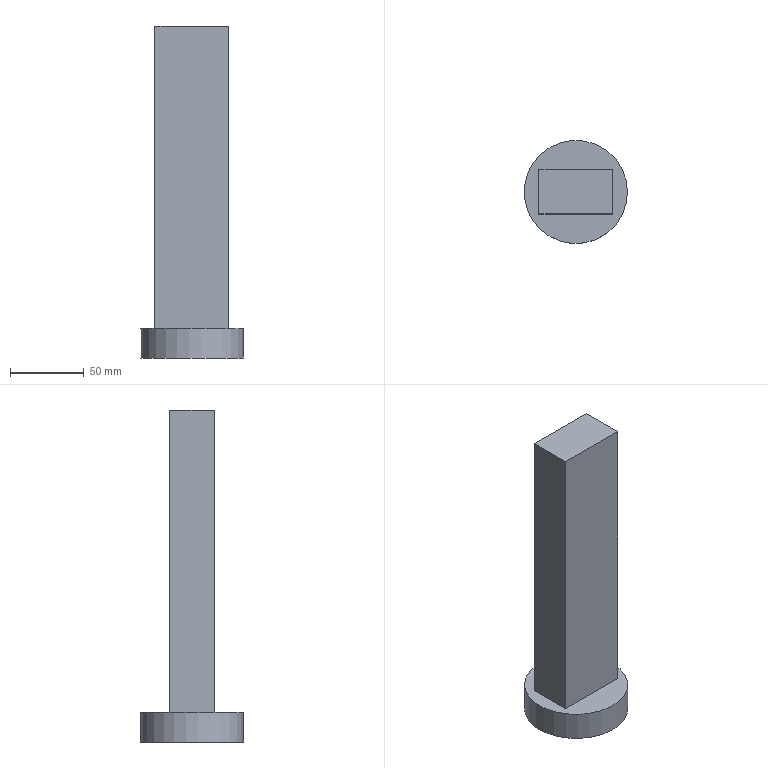Part | NX | features solid 2 | 1 solid | 8 faces | box 70 x 70 x 225 mm | volume 384469 mm3 | plane 7 | cylinder 1 | commonest cylinder face diameters 70 x1
STEP:
#1=CARTESIAN_POINT('',(980.,-425.,0.));
#2=VERTEX_POINT('',#1);
#3=CARTESIAN_POINT('',(945.,-425.,0.));
#4=DIRECTION('',(0.,0.,1.));
#5=DIRECTION('',(1.,0.,0.));
#6=AXIS2_PLACEMENT_3D('',#3,#4,#5);
#7=CIRCLE('',#6,35.);
#8=EDGE_CURVE('',#2,#2,#7,.T.);
#9=ORIENTED_EDGE('',*,*,#8,.F.);
#10=EDGE_LOOP('',(#9));
#11=FACE_BOUND('',#10,.T.);
#12=CARTESIAN_POINT('',(985.,-425.,0.));
#13=DIRECTION('',(0.,0.,1.));
#14=DIRECTION('',(1.,0.,0.));
#15=AXIS2_PLACEMENT_3D('',#12,#13,#14);
#16=PLANE('',#15);
#17=ADVANCED_FACE('',(#11),#16,.F.);
#18=ORIENTED_EDGE('',*,*,#8,.T.);
#19=EDGE_LOOP('',(#18));
#20=FACE_BOUND('',#19,.T.);
#21=CARTESIAN_POINT('',(980.,-425.,20.));
#22=VERTEX_POINT('',#21);
#23=CARTESIAN_POINT('',(945.,-425.,20.));
#24=DIRECTION('',(0.,0.,1.));
#25=DIRECTION('',(1.,0.,0.));
#26=AXIS2_PLACEMENT_3D('',#23,#24,#25);
#27=CIRCLE('',#26,35.);
#28=EDGE_CURVE('',#22,#22,#27,.T.);
#29=ORIENTED_EDGE('',*,*,#28,.F.);
#30=EDGE_LOOP('',(#29));
#31=FACE_BOUND('',#30,.T.);
#32=CARTESIAN_POINT('',(945.,-425.,30.));
#33=DIRECTION('',(0.,0.,1.));
#34=DIRECTION('',(1.,0.,0.));
#35=AXIS2_PLACEMENT_3D('',#32,#33,#34);
#36=CYLINDRICAL_SURFACE('',#35,35.);
#37=ADVANCED_FACE('',(#20,#31),#36,.T.);
#38=ORIENTED_EDGE('',*,*,#28,.T.);
#39=EDGE_LOOP('',(#38));
#40=FACE_BOUND('',#39,.T.);
#41=CARTESIAN_POINT('',(970.,-410.,20.));
#42=VERTEX_POINT('',#41);
#43=CARTESIAN_POINT('',(970.,-440.,20.));
#44=VERTEX_POINT('',#43);
#45=CARTESIAN_POINT('',(970.,-425.,20.));
#46=DIRECTION('',(0.,-1.,0.));
#47=VECTOR('',#46,1000.);
#48=LINE('',#45,#47);
#49=EDGE_CURVE('',#42,#44,#48,.T.);
#50=ORIENTED_EDGE('',*,*,#49,.T.);
#51=CARTESIAN_POINT('',(920.,-440.,20.));
#52=VERTEX_POINT('',#51);
#53=CARTESIAN_POINT('',(525.,-440.,20.));
#54=DIRECTION('',(-1.,0.,0.));
#55=VECTOR('',#54,1000.);
#56=LINE('',#53,#55);
#57=EDGE_CURVE('',#44,#52,#56,.T.);
#58=ORIENTED_EDGE('',*,*,#57,.T.);
#59=CARTESIAN_POINT('',(920.,-410.,20.));
#60=VERTEX_POINT('',#59);
#61=CARTESIAN_POINT('',(920.,-410.,20.));
#62=DIRECTION('',(0.,-1.,0.));
#63=VECTOR('',#62,1000.);
#64=LINE('',#61,#63);
#65=EDGE_CURVE('',#60,#52,#64,.T.);
#66=ORIENTED_EDGE('',*,*,#65,.F.);
#67=CARTESIAN_POINT('',(525.,-410.,20.));
#68=DIRECTION('',(-1.,0.,0.));
#69=VECTOR('',#68,1000.);
#70=LINE('',#67,#69);
#71=EDGE_CURVE('',#42,#60,#70,.T.);
#72=ORIENTED_EDGE('',*,*,#71,.F.);
#73=EDGE_LOOP('',(#50,#58,#66,#72));
#74=FACE_BOUND('',#73,.T.);
#75=CARTESIAN_POINT('',(985.,-425.,20.));
#76=DIRECTION('',(0.,0.,1.));
#77=DIRECTION('',(1.,0.,0.));
#78=AXIS2_PLACEMENT_3D('',#75,#76,#77);
#79=PLANE('',#78);
#80=ADVANCED_FACE('',(#40,#74),#79,.T.);
#81=CARTESIAN_POINT('',(970.,-410.,225.));
#82=VERTEX_POINT('',#81);
#83=CARTESIAN_POINT('',(970.,-410.,155.));
#84=DIRECTION('',(0.,0.,-1.));
#85=VECTOR('',#84,1000.);
#86=LINE('',#83,#85);
#87=EDGE_CURVE('',#82,#42,#86,.T.);
#88=ORIENTED_EDGE('',*,*,#87,.F.);
#89=CARTESIAN_POINT('',(970.,-440.,225.));
#90=VERTEX_POINT('',#89);
#91=CARTESIAN_POINT('',(970.,-410.,225.));
#92=DIRECTION('',(0.,-1.,0.));
#93=VECTOR('',#92,1000.);
#94=LINE('',#91,#93);
#95=EDGE_CURVE('',#82,#90,#94,.T.);
#96=ORIENTED_EDGE('',*,*,#95,.T.);
#97=CARTESIAN_POINT('',(970.,-440.,155.));
#98=DIRECTION('',(0.,0.,-1.));
#99=VECTOR('',#98,1000.);
#100=LINE('',#97,#99);
#101=EDGE_CURVE('',#90,#44,#100,.T.);
#102=ORIENTED_EDGE('',*,*,#101,.T.);
#103=ORIENTED_EDGE('',*,*,#49,.F.);
#104=EDGE_LOOP('',(#88,#96,#102,#103));
#105=FACE_BOUND('',#104,.T.);
#106=CARTESIAN_POINT('',(970.,-410.,365.));
#107=DIRECTION('',(-1.,0.,0.));
#108=DIRECTION('',(0.,-1.,0.));
#109=AXIS2_PLACEMENT_3D('',#106,#107,#108);
#110=PLANE('',#109);
#111=ADVANCED_FACE('',(#105),#110,.F.);
#112=CARTESIAN_POINT('',(920.,-440.,225.));
#113=VERTEX_POINT('',#112);
#114=CARTESIAN_POINT('',(920.,-440.,325.));
#115=DIRECTION('',(0.,0.,-1.));
#116=VECTOR('',#115,1000.);
#117=LINE('',#114,#116);
#118=EDGE_CURVE('',#113,#52,#117,.T.);
#119=ORIENTED_EDGE('',*,*,#118,.F.);
#120=CARTESIAN_POINT('',(920.,-410.,225.));
#121=VERTEX_POINT('',#120);
#122=CARTESIAN_POINT('',(920.,-610.,225.));
#123=DIRECTION('',(0.,1.,0.));
#124=VECTOR('',#123,1000.);
#125=LINE('',#122,#124);
#126=EDGE_CURVE('',#121,#113,#125,.F.);
#127=ORIENTED_EDGE('',*,*,#126,.F.);
#128=CARTESIAN_POINT('',(920.,-410.,325.));
#129=DIRECTION('',(0.,0.,-1.));
#130=VECTOR('',#129,1000.);
#131=LINE('',#128,#130);
#132=EDGE_CURVE('',#121,#60,#131,.T.);
#133=ORIENTED_EDGE('',*,*,#132,.T.);
#134=ORIENTED_EDGE('',*,*,#65,.T.);
#135=EDGE_LOOP('',(#119,#127,#133,#134));
#136=FACE_BOUND('',#135,.T.);
#137=CARTESIAN_POINT('',(920.,-410.,325.));
#138=DIRECTION('',(1.,0.,0.));
#139=DIRECTION('',(0.,0.,-1.));
#140=AXIS2_PLACEMENT_3D('',#137,#138,#139);
#141=PLANE('',#140);
#142=ADVANCED_FACE('',(#136),#141,.F.);
#143=CARTESIAN_POINT('',(540.,-440.,225.));
#144=DIRECTION('',(1.,0.,0.));
#145=VECTOR('',#144,1000.);
#146=LINE('',#143,#145);
#147=EDGE_CURVE('',#113,#90,#146,.T.);
#148=ORIENTED_EDGE('',*,*,#147,.F.);
#149=ORIENTED_EDGE('',*,*,#118,.T.);
#150=ORIENTED_EDGE('',*,*,#57,.F.);
#151=ORIENTED_EDGE('',*,*,#101,.F.);
#152=EDGE_LOOP('',(#148,#149,#150,#151));
#153=FACE_BOUND('',#152,.T.);
#154=CARTESIAN_POINT('',(540.,-440.,155.));
#155=DIRECTION('',(0.,-1.,0.));
#156=DIRECTION('',(0.,0.,-1.));
#157=AXIS2_PLACEMENT_3D('',#154,#155,#156);
#158=PLANE('',#157);
#159=ADVANCED_FACE('',(#153),#158,.T.);
#160=ORIENTED_EDGE('',*,*,#132,.F.);
#161=CARTESIAN_POINT('',(540.,-410.,225.));
#162=DIRECTION('',(1.,0.,0.));
#163=VECTOR('',#162,1000.);
#164=LINE('',#161,#163);
#165=EDGE_CURVE('',#121,#82,#164,.T.);
#166=ORIENTED_EDGE('',*,*,#165,.T.);
#167=ORIENTED_EDGE('',*,*,#87,.T.);
#168=ORIENTED_EDGE('',*,*,#71,.T.);
#169=EDGE_LOOP('',(#160,#166,#167,#168));
#170=FACE_BOUND('',#169,.T.);
#171=CARTESIAN_POINT('',(540.,-410.,155.));
#172=DIRECTION('',(0.,-1.,0.));
#173=DIRECTION('',(0.,0.,-1.));
#174=AXIS2_PLACEMENT_3D('',#171,#172,#173);
#175=PLANE('',#174);
#176=ADVANCED_FACE('',(#170),#175,.F.);
#177=ORIENTED_EDGE('',*,*,#165,.F.);
#178=ORIENTED_EDGE('',*,*,#126,.T.);
#179=ORIENTED_EDGE('',*,*,#147,.T.);
#180=ORIENTED_EDGE('',*,*,#95,.F.);
#181=EDGE_LOOP('',(#177,#178,#179,#180));
#182=FACE_BOUND('',#181,.T.);
#183=CARTESIAN_POINT('',(-620.,-610.,225.));
#184=DIRECTION('',(0.,0.,-1.));
#185=DIRECTION('',(-1.,0.,0.));
#186=AXIS2_PLACEMENT_3D('',#183,#184,#185);
#187=PLANE('',#186);
#188=ADVANCED_FACE('',(#182),#187,.F.);
#189=CLOSED_SHELL('',(#17,#37,#80,#111,#142,#159,#176,#188));
#190=MANIFOLD_SOLID_BREP('',#189);
#191=(LENGTH_UNIT()NAMED_UNIT(*)SI_UNIT(.MILLI.,.METRE.));
#192=UNCERTAINTY_MEASURE_WITH_UNIT(LENGTH_MEASURE(0.00001),#191,'','');
#193=(NAMED_UNIT(*)PLANE_ANGLE_UNIT()SI_UNIT($,.RADIAN.));
#194=(NAMED_UNIT(*)SI_UNIT($,.STERADIAN.)SOLID_ANGLE_UNIT());
#195=(GEOMETRIC_REPRESENTATION_CONTEXT(3)GLOBAL_UNCERTAINTY_ASSIGNED_CONTEXT((#192))GLOBAL_UNIT_ASSIGNED_CONTEXT((#191,#193,#194))REPRESENTATION_CONTEXT('',''));
#196=ADVANCED_BREP_SHAPE_REPRESENTATION('',(#190),#195);